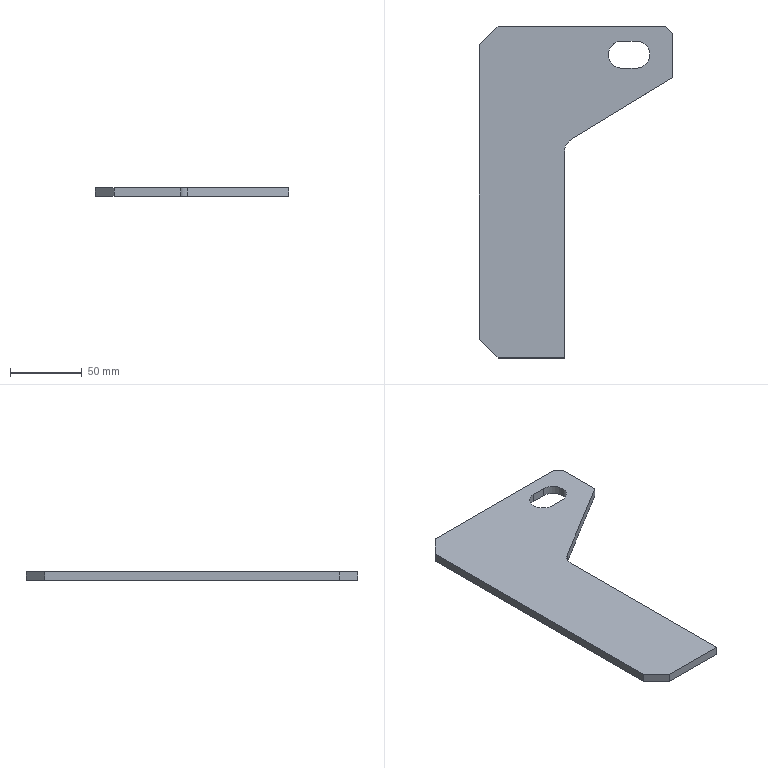Part | STEP file | 筋Plate-250×125-5 | 1 solid | 17 faces | box 135 x 232 x 6 mm | volume 105651 mm3 | plane 13 | cylinder 4 | commonest cylinder face diameters 19 x3 20 x1
STEP:
#1=CARTESIAN_POINT('',(0.,0.,0.));
#2=DIRECTION('',(0.,0.,1.));
#3=DIRECTION('',(1.,0.,0.));
#4=AXIS2_PLACEMENT_3D('',#1,#2,#3);
#5=CARTESIAN_POINT('',(32.,105.5,3.));
#6=VERTEX_POINT('',#5);
#7=CARTESIAN_POINT('',(32.,105.5,-3.));
#8=VERTEX_POINT('',#7);
#9=CARTESIAN_POINT('',(32.,105.5,-3.));
#10=DIRECTION('',(0.,0.,-1.));
#11=VECTOR('',#10,1.);
#12=LINE('',#9,#11);
#13=CARTESIAN_POINT('',(32.,96.,-3.));
#14=DIRECTION('',(0.,0.,-1.));
#15=DIRECTION('',(-1.,0.,0.));
#16=AXIS2_PLACEMENT_3D('',#13,#14,#15);
#17=CYLINDRICAL_SURFACE('',#16,9.5);
#18=CARTESIAN_POINT('',(1.571,0.));
#19=DIRECTION('',(0.,1.));
#20=VECTOR('',#19,1.);
#21=LINE('',#18,#20);
#22=(GEOMETRIC_REPRESENTATION_CONTEXT(2)PARAMETRIC_REPRESENTATION_CONTEXT()REPRESENTATION_CONTEXT('',''));
#23=DEFINITIONAL_REPRESENTATION('',(#21),#22);
#24=PCURVE('',#17,#23);
#25=CARTESIAN_POINT('',(42.,105.5,-3.));
#26=DIRECTION('',(0.,1.,0.));
#27=DIRECTION('',(0.,0.,1.));
#28=AXIS2_PLACEMENT_3D('',#25,#26,#27);
#29=PLANE('',#28);
#30=CARTESIAN_POINT('',(0.,-10.));
#31=DIRECTION('',(-1.,0.));
#32=VECTOR('',#31,1.);
#33=LINE('',#30,#32);
#34=(GEOMETRIC_REPRESENTATION_CONTEXT(2)PARAMETRIC_REPRESENTATION_CONTEXT()REPRESENTATION_CONTEXT('',''));
#35=DEFINITIONAL_REPRESENTATION('',(#33),#34);
#36=PCURVE('',#29,#35);
#37=SURFACE_CURVE('',#12,(#24,#36),.PCURVE_S1.);
#38=EDGE_CURVE('',#6,#8,#37,.T.);
#39=ORIENTED_EDGE('',*,*,#38,.T.);
#40=CARTESIAN_POINT('',(22.5,96.,-3.));
#41=VERTEX_POINT('',#40);
#42=CARTESIAN_POINT('',(32.,96.,-3.));
#43=DIRECTION('',(0.,0.,-1.));
#44=DIRECTION('',(-1.,0.,0.));
#45=AXIS2_PLACEMENT_3D('',#42,#43,#44);
#46=CIRCLE('',#45,9.5);
#47=CARTESIAN_POINT('',(0.,0.));
#48=DIRECTION('',(1.,0.));
#49=VECTOR('',#48,1.);
#50=LINE('',#47,#49);
#51=(GEOMETRIC_REPRESENTATION_CONTEXT(2)PARAMETRIC_REPRESENTATION_CONTEXT()REPRESENTATION_CONTEXT('',''));
#52=DEFINITIONAL_REPRESENTATION('',(#50),#51);
#53=PCURVE('',#17,#52);
#54=CARTESIAN_POINT('',(0.,0.,-3.));
#55=DIRECTION('',(0.,0.,1.));
#56=DIRECTION('',(1.,0.,0.));
#57=AXIS2_PLACEMENT_3D('',#54,#55,#56);
#58=PLANE('',#57);
#59=CARTESIAN_POINT('',(22.5,96.));
#60=CARTESIAN_POINT('',(22.5,112.454));
#61=CARTESIAN_POINT('',(36.75,104.227));
#62=CARTESIAN_POINT('',(51.,96.));
#63=CARTESIAN_POINT('',(36.75,87.773));
#64=CARTESIAN_POINT('',(22.5,79.546));
#65=CARTESIAN_POINT('',(22.5,96.));
#66=(BOUNDED_CURVE()B_SPLINE_CURVE(2,(#59,#60,#61,#62,#63,#64,#65),.UNSPECIFIED.,.T.,.F.)B_SPLINE_CURVE_WITH_KNOTS((1,2,2,2,2,1),(-2.094,0.,2.094,4.189,6.283,8.378),.UNSPECIFIED.)CURVE()GEOMETRIC_REPRESENTATION_ITEM()RATIONAL_B_SPLINE_CURVE((1.,0.5,1.,0.5,1.,0.5,1.))REPRESENTATION_ITEM(''));
#67=(GEOMETRIC_REPRESENTATION_CONTEXT(2)PARAMETRIC_REPRESENTATION_CONTEXT()REPRESENTATION_CONTEXT('',''));
#68=DEFINITIONAL_REPRESENTATION('',(#66),#67);
#69=PCURVE('',#58,#68);
#70=SURFACE_CURVE('',#46,(#53,#69),.PCURVE_S1.);
#71=EDGE_CURVE('',#41,#8,#70,.T.);
#72=ORIENTED_EDGE('',*,*,#71,.F.);
#73=CARTESIAN_POINT('',(22.5,96.,3.));
#74=VERTEX_POINT('',#73);
#75=CARTESIAN_POINT('',(22.5,96.,-3.));
#76=DIRECTION('',(0.,0.,-1.));
#77=VECTOR('',#76,1.);
#78=LINE('',#75,#77);
#79=CARTESIAN_POINT('',(0.,0.));
#80=DIRECTION('',(0.,1.));
#81=VECTOR('',#80,1.);
#82=LINE('',#79,#81);
#83=(GEOMETRIC_REPRESENTATION_CONTEXT(2)PARAMETRIC_REPRESENTATION_CONTEXT()REPRESENTATION_CONTEXT('',''));
#84=DEFINITIONAL_REPRESENTATION('',(#82),#83);
#85=PCURVE('',#17,#84);
#86=CARTESIAN_POINT('',(32.,96.,-3.));
#87=DIRECTION('',(0.,0.,-1.));
#88=DIRECTION('',(-1.,0.,0.));
#89=AXIS2_PLACEMENT_3D('',#86,#87,#88);
#90=CYLINDRICAL_SURFACE('',#89,9.5);
#91=CARTESIAN_POINT('',(6.283,0.));
#92=DIRECTION('',(0.,1.));
#93=VECTOR('',#92,1.);
#94=LINE('',#91,#93);
#95=(GEOMETRIC_REPRESENTATION_CONTEXT(2)PARAMETRIC_REPRESENTATION_CONTEXT()REPRESENTATION_CONTEXT('',''));
#96=DEFINITIONAL_REPRESENTATION('',(#94),#95);
#97=PCURVE('',#90,#96);
#98=SURFACE_CURVE('',#78,(#85,#97),.PCURVE_S1.);
#99=EDGE_CURVE('',#74,#41,#98,.T.);
#100=ORIENTED_EDGE('',*,*,#99,.F.);
#101=CARTESIAN_POINT('',(32.,96.,3.));
#102=DIRECTION('',(0.,0.,1.));
#103=DIRECTION('',(1.,0.,0.));
#104=AXIS2_PLACEMENT_3D('',#101,#102,#103);
#105=CIRCLE('',#104,9.5);
#106=CARTESIAN_POINT('',(3.142,-6.));
#107=DIRECTION('',(-1.,0.));
#108=VECTOR('',#107,1.);
#109=LINE('',#106,#108);
#110=(GEOMETRIC_REPRESENTATION_CONTEXT(2)PARAMETRIC_REPRESENTATION_CONTEXT()REPRESENTATION_CONTEXT('',''));
#111=DEFINITIONAL_REPRESENTATION('',(#109),#110);
#112=PCURVE('',#17,#111);
#113=CARTESIAN_POINT('',(0.,0.,3.));
#114=DIRECTION('',(0.,0.,1.));
#115=DIRECTION('',(1.,0.,0.));
#116=AXIS2_PLACEMENT_3D('',#113,#114,#115);
#117=PLANE('',#116);
#118=CARTESIAN_POINT('',(32.,96.));
#119=DIRECTION('',(1.,0.));
#120=AXIS2_PLACEMENT_2D('',#118,#119);
#121=CIRCLE('',#120,9.5);
#122=(GEOMETRIC_REPRESENTATION_CONTEXT(2)PARAMETRIC_REPRESENTATION_CONTEXT()REPRESENTATION_CONTEXT('',''));
#123=DEFINITIONAL_REPRESENTATION('',(#121),#122);
#124=PCURVE('',#117,#123);
#125=SURFACE_CURVE('',#105,(#112,#124),.PCURVE_S1.);
#126=EDGE_CURVE('',#6,#74,#125,.T.);
#127=ORIENTED_EDGE('',*,*,#126,.F.);
#128=EDGE_LOOP('',(#39,#72,#100,#127));
#129=FACE_BOUND('',#128,.F.);
#130=ADVANCED_FACE('',(#129),#17,.F.);
#131=CARTESIAN_POINT('',(67.5,80.,-3.));
#132=VERTEX_POINT('',#131);
#133=CARTESIAN_POINT('',(67.5,111.,-3.));
#134=VERTEX_POINT('',#133);
#135=CARTESIAN_POINT('',(67.5,116.,-3.));
#136=DIRECTION('',(0.,1.,0.));
#137=VECTOR('',#136,1.);
#138=LINE('',#135,#137);
#139=CARTESIAN_POINT('',(67.5,116.,3.));
#140=DIRECTION('',(-1.,0.,0.));
#141=DIRECTION('',(0.,-1.,0.));
#142=AXIS2_PLACEMENT_3D('',#139,#140,#141);
#143=PLANE('',#142);
#144=CARTESIAN_POINT('',(0.,-6.));
#145=DIRECTION('',(-1.,0.));
#146=VECTOR('',#145,1.);
#147=LINE('',#144,#146);
#148=(GEOMETRIC_REPRESENTATION_CONTEXT(2)PARAMETRIC_REPRESENTATION_CONTEXT()REPRESENTATION_CONTEXT('',''));
#149=DEFINITIONAL_REPRESENTATION('',(#147),#148);
#150=PCURVE('',#143,#149);
#151=CARTESIAN_POINT('',(67.5,116.));
#152=DIRECTION('',(0.,1.));
#153=VECTOR('',#152,1.);
#154=LINE('',#151,#153);
#155=(GEOMETRIC_REPRESENTATION_CONTEXT(2)PARAMETRIC_REPRESENTATION_CONTEXT()REPRESENTATION_CONTEXT('',''));
#156=DEFINITIONAL_REPRESENTATION('',(#154),#155);
#157=PCURVE('',#58,#156);
#158=SURFACE_CURVE('',#138,(#150,#157),.PCURVE_S1.);
#159=EDGE_CURVE('',#132,#134,#158,.T.);
#160=ORIENTED_EDGE('',*,*,#159,.T.);
#161=CARTESIAN_POINT('',(67.5,111.,3.));
#162=VERTEX_POINT('',#161);
#163=CARTESIAN_POINT('',(67.5,111.,3.));
#164=DIRECTION('',(0.,0.,1.));
#165=VECTOR('',#164,1.);
#166=LINE('',#163,#165);
#167=CARTESIAN_POINT('',(5.,0.));
#168=DIRECTION('',(0.,1.));
#169=VECTOR('',#168,1.);
#170=LINE('',#167,#169);
#171=(GEOMETRIC_REPRESENTATION_CONTEXT(2)PARAMETRIC_REPRESENTATION_CONTEXT()REPRESENTATION_CONTEXT('',''));
#172=DEFINITIONAL_REPRESENTATION('',(#170),#171);
#173=PCURVE('',#143,#172);
#174=CARTESIAN_POINT('',(62.5,116.,3.));
#175=DIRECTION('',(-0.7071,-0.7071,0.));
#176=DIRECTION('',(0.,0.,-1.));
#177=AXIS2_PLACEMENT_3D('',#174,#175,#176);
#178=PLANE('',#177);
#179=CARTESIAN_POINT('',(0.,7.071));
#180=DIRECTION('',(-1.,0.));
#181=VECTOR('',#180,1.);
#182=LINE('',#179,#181);
#183=(GEOMETRIC_REPRESENTATION_CONTEXT(2)PARAMETRIC_REPRESENTATION_CONTEXT()REPRESENTATION_CONTEXT('',''));
#184=DEFINITIONAL_REPRESENTATION('',(#182),#183);
#185=PCURVE('',#178,#184);
#186=SURFACE_CURVE('',#166,(#173,#185),.PCURVE_S1.);
#187=EDGE_CURVE('',#134,#162,#186,.T.);
#188=ORIENTED_EDGE('',*,*,#187,.T.);
#189=CARTESIAN_POINT('',(67.5,80.,3.));
#190=VERTEX_POINT('',#189);
#191=CARTESIAN_POINT('',(67.5,116.,3.));
#192=DIRECTION('',(0.,1.,0.));
#193=VECTOR('',#192,1.);
#194=LINE('',#191,#193);
#195=CARTESIAN_POINT('',(0.,0.));
#196=DIRECTION('',(-1.,0.));
#197=VECTOR('',#196,1.);
#198=LINE('',#195,#197);
#199=(GEOMETRIC_REPRESENTATION_CONTEXT(2)PARAMETRIC_REPRESENTATION_CONTEXT()REPRESENTATION_CONTEXT('',''));
#200=DEFINITIONAL_REPRESENTATION('',(#198),#199);
#201=PCURVE('',#143,#200);
#202=CARTESIAN_POINT('',(67.5,116.));
#203=DIRECTION('',(0.,1.));
#204=VECTOR('',#203,1.);
#205=LINE('',#202,#204);
#206=(GEOMETRIC_REPRESENTATION_CONTEXT(2)PARAMETRIC_REPRESENTATION_CONTEXT()REPRESENTATION_CONTEXT('',''));
#207=DEFINITIONAL_REPRESENTATION('',(#205),#206);
#208=PCURVE('',#117,#207);
#209=SURFACE_CURVE('',#194,(#201,#208),.PCURVE_S1.);
#210=EDGE_CURVE('',#190,#162,#209,.T.);
#211=ORIENTED_EDGE('',*,*,#210,.F.);
#212=CARTESIAN_POINT('',(67.5,80.,-3.));
#213=DIRECTION('',(0.,0.,1.));
#214=VECTOR('',#213,1.);
#215=LINE('',#212,#214);
#216=CARTESIAN_POINT('',(36.,-6.));
#217=DIRECTION('',(0.,1.));
#218=VECTOR('',#217,1.);
#219=LINE('',#216,#218);
#220=(GEOMETRIC_REPRESENTATION_CONTEXT(2)PARAMETRIC_REPRESENTATION_CONTEXT()REPRESENTATION_CONTEXT('',''));
#221=DEFINITIONAL_REPRESENTATION('',(#219),#220);
#222=PCURVE('',#143,#221);
#223=CARTESIAN_POINT('',(67.5,80.,-3.));
#224=DIRECTION('',(-0.5203,0.854,0.));
#225=DIRECTION('',(-0.854,-0.5203,0.));
#226=AXIS2_PLACEMENT_3D('',#223,#224,#225);
#227=PLANE('',#226);
#228=CARTESIAN_POINT('',(0.,0.));
#229=DIRECTION('',(0.,1.));
#230=VECTOR('',#229,1.);
#231=LINE('',#228,#230);
#232=(GEOMETRIC_REPRESENTATION_CONTEXT(2)PARAMETRIC_REPRESENTATION_CONTEXT()REPRESENTATION_CONTEXT('',''));
#233=DEFINITIONAL_REPRESENTATION('',(#231),#232);
#234=PCURVE('',#227,#233);
#235=SURFACE_CURVE('',#215,(#222,#234),.PCURVE_S1.);
#236=EDGE_CURVE('',#132,#190,#235,.T.);
#237=ORIENTED_EDGE('',*,*,#236,.F.);
#238=EDGE_LOOP('',(#160,#188,#211,#237));
#239=FACE_BOUND('',#238,.T.);
#240=ADVANCED_FACE('',(#239),#143,.F.);
#241=CARTESIAN_POINT('',(62.5,116.,3.));
#242=VERTEX_POINT('',#241);
#243=CARTESIAN_POINT('',(-54.5,116.,3.));
#244=VERTEX_POINT('',#243);
#245=CARTESIAN_POINT('',(-67.5,116.,3.));
#246=DIRECTION('',(-1.,0.,0.));
#247=VECTOR('',#246,1.);
#248=LINE('',#245,#247);
#249=CARTESIAN_POINT('',(-67.5,116.,3.));
#250=DIRECTION('',(0.,-1.,0.));
#251=DIRECTION('',(0.,0.,-1.));
#252=AXIS2_PLACEMENT_3D('',#249,#250,#251);
#253=PLANE('',#252);
#254=CARTESIAN_POINT('',(0.,0.));
#255=DIRECTION('',(0.,-1.));
#256=VECTOR('',#255,1.);
#257=LINE('',#254,#256);
#258=(GEOMETRIC_REPRESENTATION_CONTEXT(2)PARAMETRIC_REPRESENTATION_CONTEXT()REPRESENTATION_CONTEXT('',''));
#259=DEFINITIONAL_REPRESENTATION('',(#257),#258);
#260=PCURVE('',#253,#259);
#261=CARTESIAN_POINT('',(-67.5,116.));
#262=DIRECTION('',(-1.,0.));
#263=VECTOR('',#262,1.);
#264=LINE('',#261,#263);
#265=(GEOMETRIC_REPRESENTATION_CONTEXT(2)PARAMETRIC_REPRESENTATION_CONTEXT()REPRESENTATION_CONTEXT('',''));
#266=DEFINITIONAL_REPRESENTATION('',(#264),#265);
#267=PCURVE('',#117,#266);
#268=SURFACE_CURVE('',#248,(#260,#267),.PCURVE_S1.);
#269=EDGE_CURVE('',#242,#244,#268,.T.);
#270=ORIENTED_EDGE('',*,*,#269,.F.);
#271=CARTESIAN_POINT('',(62.5,116.,-3.));
#272=VERTEX_POINT('',#271);
#273=CARTESIAN_POINT('',(62.5,116.,3.));
#274=DIRECTION('',(0.,0.,-1.));
#275=VECTOR('',#274,1.);
#276=LINE('',#273,#275);
#277=CARTESIAN_POINT('',(0.,130.));
#278=DIRECTION('',(1.,0.));
#279=VECTOR('',#278,1.);
#280=LINE('',#277,#279);
#281=(GEOMETRIC_REPRESENTATION_CONTEXT(2)PARAMETRIC_REPRESENTATION_CONTEXT()REPRESENTATION_CONTEXT('',''));
#282=DEFINITIONAL_REPRESENTATION('',(#280),#281);
#283=PCURVE('',#253,#282);
#284=CARTESIAN_POINT('',(0.,0.));
#285=DIRECTION('',(1.,0.));
#286=VECTOR('',#285,1.);
#287=LINE('',#284,#286);
#288=(GEOMETRIC_REPRESENTATION_CONTEXT(2)PARAMETRIC_REPRESENTATION_CONTEXT()REPRESENTATION_CONTEXT('',''));
#289=DEFINITIONAL_REPRESENTATION('',(#287),#288);
#290=PCURVE('',#178,#289);
#291=SURFACE_CURVE('',#276,(#283,#290),.PCURVE_S1.);
#292=EDGE_CURVE('',#242,#272,#291,.T.);
#293=ORIENTED_EDGE('',*,*,#292,.T.);
#294=CARTESIAN_POINT('',(-54.5,116.,-3.));
#295=VERTEX_POINT('',#294);
#296=CARTESIAN_POINT('',(-67.5,116.,-3.));
#297=DIRECTION('',(-1.,0.,0.));
#298=VECTOR('',#297,1.);
#299=LINE('',#296,#298);
#300=CARTESIAN_POINT('',(6.,0.));
#301=DIRECTION('',(0.,-1.));
#302=VECTOR('',#301,1.);
#303=LINE('',#300,#302);
#304=(GEOMETRIC_REPRESENTATION_CONTEXT(2)PARAMETRIC_REPRESENTATION_CONTEXT()REPRESENTATION_CONTEXT('',''));
#305=DEFINITIONAL_REPRESENTATION('',(#303),#304);
#306=PCURVE('',#253,#305);
#307=CARTESIAN_POINT('',(-67.5,116.));
#308=DIRECTION('',(-1.,0.));
#309=VECTOR('',#308,1.);
#310=LINE('',#307,#309);
#311=(GEOMETRIC_REPRESENTATION_CONTEXT(2)PARAMETRIC_REPRESENTATION_CONTEXT()REPRESENTATION_CONTEXT('',''));
#312=DEFINITIONAL_REPRESENTATION('',(#310),#311);
#313=PCURVE('',#58,#312);
#314=SURFACE_CURVE('',#299,(#306,#313),.PCURVE_S1.);
#315=EDGE_CURVE('',#272,#295,#314,.T.);
#316=ORIENTED_EDGE('',*,*,#315,.T.);
#317=CARTESIAN_POINT('',(-54.5,116.,3.));
#318=DIRECTION('',(0.,0.,1.));
#319=VECTOR('',#318,1.);
#320=LINE('',#317,#319);
#321=CARTESIAN_POINT('',(0.,13.));
#322=DIRECTION('',(-1.,0.));
#323=VECTOR('',#322,1.);
#324=LINE('',#321,#323);
#325=(GEOMETRIC_REPRESENTATION_CONTEXT(2)PARAMETRIC_REPRESENTATION_CONTEXT()REPRESENTATION_CONTEXT('',''));
#326=DEFINITIONAL_REPRESENTATION('',(#324),#325);
#327=PCURVE('',#253,#326);
#328=CARTESIAN_POINT('',(-67.5,103.,3.));
#329=DIRECTION('',(0.7071,-0.7071,0.));
#330=DIRECTION('',(0.,0.,-1.));
#331=AXIS2_PLACEMENT_3D('',#328,#329,#330);
#332=PLANE('',#331);
#333=CARTESIAN_POINT('',(0.,18.385));
#334=DIRECTION('',(-1.,0.));
#335=VECTOR('',#334,1.);
#336=LINE('',#333,#335);
#337=(GEOMETRIC_REPRESENTATION_CONTEXT(2)PARAMETRIC_REPRESENTATION_CONTEXT()REPRESENTATION_CONTEXT('',''));
#338=DEFINITIONAL_REPRESENTATION('',(#336),#337);
#339=PCURVE('',#332,#338);
#340=SURFACE_CURVE('',#320,(#327,#339),.PCURVE_S1.);
#341=EDGE_CURVE('',#295,#244,#340,.T.);
#342=ORIENTED_EDGE('',*,*,#341,.T.);
#343=EDGE_LOOP('',(#270,#293,#316,#342));
#344=FACE_BOUND('',#343,.T.);
#345=ADVANCED_FACE('',(#344),#253,.F.);
#346=CARTESIAN_POINT('',(-67.5,103.,-3.));
#347=VERTEX_POINT('',#346);
#348=CARTESIAN_POINT('',(-67.5,-103.,-3.));
#349=VERTEX_POINT('',#348);
#350=CARTESIAN_POINT('',(-67.5,116.,-3.));
#351=DIRECTION('',(0.,-1.,0.));
#352=VECTOR('',#351,1.);
#353=LINE('',#350,#352);
#354=CARTESIAN_POINT('',(-67.5,116.,3.));
#355=DIRECTION('',(1.,0.,0.));
#356=DIRECTION('',(0.,1.,0.));
#357=AXIS2_PLACEMENT_3D('',#354,#355,#356);
#358=PLANE('',#357);
#359=CARTESIAN_POINT('',(0.,-6.));
#360=DIRECTION('',(-1.,0.));
#361=VECTOR('',#360,1.);
#362=LINE('',#359,#361);
#363=(GEOMETRIC_REPRESENTATION_CONTEXT(2)PARAMETRIC_REPRESENTATION_CONTEXT()REPRESENTATION_CONTEXT('',''));
#364=DEFINITIONAL_REPRESENTATION('',(#362),#363);
#365=PCURVE('',#358,#364);
#366=CARTESIAN_POINT('',(-67.5,116.));
#367=DIRECTION('',(0.,-1.));
#368=VECTOR('',#367,1.);
#369=LINE('',#366,#368);
#370=(GEOMETRIC_REPRESENTATION_CONTEXT(2)PARAMETRIC_REPRESENTATION_CONTEXT()REPRESENTATION_CONTEXT('',''));
#371=DEFINITIONAL_REPRESENTATION('',(#369),#370);
#372=PCURVE('',#58,#371);
#373=SURFACE_CURVE('',#353,(#365,#372),.PCURVE_S1.);
#374=EDGE_CURVE('',#347,#349,#373,.T.);
#375=ORIENTED_EDGE('',*,*,#374,.T.);
#376=CARTESIAN_POINT('',(-67.5,-103.,3.));
#377=VERTEX_POINT('',#376);
#378=CARTESIAN_POINT('',(-67.5,-103.,3.));
#379=DIRECTION('',(0.,0.,1.));
#380=VECTOR('',#379,1.);
#381=LINE('',#378,#380);
#382=CARTESIAN_POINT('',(-219.,0.));
#383=DIRECTION('',(0.,1.));
#384=VECTOR('',#383,1.);
#385=LINE('',#382,#384);
#386=(GEOMETRIC_REPRESENTATION_CONTEXT(2)PARAMETRIC_REPRESENTATION_CONTEXT()REPRESENTATION_CONTEXT('',''));
#387=DEFINITIONAL_REPRESENTATION('',(#385),#386);
#388=PCURVE('',#358,#387);
#389=CARTESIAN_POINT('',(-54.5,-116.,3.));
#390=DIRECTION('',(0.7071,0.7071,0.));
#391=DIRECTION('',(0.,0.,-1.));
#392=AXIS2_PLACEMENT_3D('',#389,#390,#391);
#393=PLANE('',#392);
#394=CARTESIAN_POINT('',(0.,18.385));
#395=DIRECTION('',(-1.,0.));
#396=VECTOR('',#395,1.);
#397=LINE('',#394,#396);
#398=(GEOMETRIC_REPRESENTATION_CONTEXT(2)PARAMETRIC_REPRESENTATION_CONTEXT()REPRESENTATION_CONTEXT('',''));
#399=DEFINITIONAL_REPRESENTATION('',(#397),#398);
#400=PCURVE('',#393,#399);
#401=SURFACE_CURVE('',#381,(#388,#400),.PCURVE_S1.);
#402=EDGE_CURVE('',#349,#377,#401,.T.);
#403=ORIENTED_EDGE('',*,*,#402,.T.);
#404=CARTESIAN_POINT('',(-67.5,103.,3.));
#405=VERTEX_POINT('',#404);
#406=CARTESIAN_POINT('',(-67.5,116.,3.));
#407=DIRECTION('',(0.,-1.,0.));
#408=VECTOR('',#407,1.);
#409=LINE('',#406,#408);
#410=CARTESIAN_POINT('',(0.,0.));
#411=DIRECTION('',(-1.,0.));
#412=VECTOR('',#411,1.);
#413=LINE('',#410,#412);
#414=(GEOMETRIC_REPRESENTATION_CONTEXT(2)PARAMETRIC_REPRESENTATION_CONTEXT()REPRESENTATION_CONTEXT('',''));
#415=DEFINITIONAL_REPRESENTATION('',(#413),#414);
#416=PCURVE('',#358,#415);
#417=CARTESIAN_POINT('',(-67.5,116.));
#418=DIRECTION('',(0.,-1.));
#419=VECTOR('',#418,1.);
#420=LINE('',#417,#419);
#421=(GEOMETRIC_REPRESENTATION_CONTEXT(2)PARAMETRIC_REPRESENTATION_CONTEXT()REPRESENTATION_CONTEXT('',''));
#422=DEFINITIONAL_REPRESENTATION('',(#420),#421);
#423=PCURVE('',#117,#422);
#424=SURFACE_CURVE('',#409,(#416,#423),.PCURVE_S1.);
#425=EDGE_CURVE('',#405,#377,#424,.T.);
#426=ORIENTED_EDGE('',*,*,#425,.F.);
#427=CARTESIAN_POINT('',(-67.5,103.,3.));
#428=DIRECTION('',(0.,0.,-1.));
#429=VECTOR('',#428,1.);
#430=LINE('',#427,#429);
#431=CARTESIAN_POINT('',(-13.,0.));
#432=DIRECTION('',(0.,-1.));
#433=VECTOR('',#432,1.);
#434=LINE('',#431,#433);
#435=(GEOMETRIC_REPRESENTATION_CONTEXT(2)PARAMETRIC_REPRESENTATION_CONTEXT()REPRESENTATION_CONTEXT('',''));
#436=DEFINITIONAL_REPRESENTATION('',(#434),#435);
#437=PCURVE('',#358,#436);
#438=CARTESIAN_POINT('',(0.,0.));
#439=DIRECTION('',(1.,0.));
#440=VECTOR('',#439,1.);
#441=LINE('',#438,#440);
#442=(GEOMETRIC_REPRESENTATION_CONTEXT(2)PARAMETRIC_REPRESENTATION_CONTEXT()REPRESENTATION_CONTEXT('',''));
#443=DEFINITIONAL_REPRESENTATION('',(#441),#442);
#444=PCURVE('',#332,#443);
#445=SURFACE_CURVE('',#430,(#437,#444),.PCURVE_S1.);
#446=EDGE_CURVE('',#405,#347,#445,.T.);
#447=ORIENTED_EDGE('',*,*,#446,.T.);
#448=EDGE_LOOP('',(#375,#403,#426,#447));
#449=FACE_BOUND('',#448,.T.);
#450=ADVANCED_FACE('',(#449),#358,.F.);
#451=CARTESIAN_POINT('',(-54.5,-116.,3.));
#452=VERTEX_POINT('',#451);
#453=CARTESIAN_POINT('',(-8.,-116.,3.));
#454=VERTEX_POINT('',#453);
#455=CARTESIAN_POINT('',(-67.5,-116.,3.));
#456=DIRECTION('',(1.,0.,0.));
#457=VECTOR('',#456,1.);
#458=LINE('',#455,#457);
#459=CARTESIAN_POINT('',(-67.5,-116.,3.));
#460=DIRECTION('',(0.,1.,0.));
#461=DIRECTION('',(0.,0.,1.));
#462=AXIS2_PLACEMENT_3D('',#459,#460,#461);
#463=PLANE('',#462);
#464=CARTESIAN_POINT('',(0.,0.));
#465=DIRECTION('',(0.,1.));
#466=VECTOR('',#465,1.);
#467=LINE('',#464,#466);
#468=(GEOMETRIC_REPRESENTATION_CONTEXT(2)PARAMETRIC_REPRESENTATION_CONTEXT()REPRESENTATION_CONTEXT('',''));
#469=DEFINITIONAL_REPRESENTATION('',(#467),#468);
#470=PCURVE('',#463,#469);
#471=CARTESIAN_POINT('',(-67.5,-116.));
#472=DIRECTION('',(1.,0.));
#473=VECTOR('',#472,1.);
#474=LINE('',#471,#473);
#475=(GEOMETRIC_REPRESENTATION_CONTEXT(2)PARAMETRIC_REPRESENTATION_CONTEXT()REPRESENTATION_CONTEXT('',''));
#476=DEFINITIONAL_REPRESENTATION('',(#474),#475);
#477=PCURVE('',#117,#476);
#478=SURFACE_CURVE('',#458,(#470,#477),.PCURVE_S1.);
#479=EDGE_CURVE('',#452,#454,#478,.T.);
#480=ORIENTED_EDGE('',*,*,#479,.F.);
#481=CARTESIAN_POINT('',(-54.5,-116.,-3.));
#482=VERTEX_POINT('',#481);
#483=CARTESIAN_POINT('',(-54.5,-116.,3.));
#484=DIRECTION('',(0.,0.,-1.));
#485=VECTOR('',#484,1.);
#486=LINE('',#483,#485);
#487=CARTESIAN_POINT('',(0.,13.));
#488=DIRECTION('',(-1.,0.));
#489=VECTOR('',#488,1.);
#490=LINE('',#487,#489);
#491=(GEOMETRIC_REPRESENTATION_CONTEXT(2)PARAMETRIC_REPRESENTATION_CONTEXT()REPRESENTATION_CONTEXT('',''));
#492=DEFINITIONAL_REPRESENTATION('',(#490),#491);
#493=PCURVE('',#463,#492);
#494=CARTESIAN_POINT('',(0.,0.));
#495=DIRECTION('',(1.,0.));
#496=VECTOR('',#495,1.);
#497=LINE('',#494,#496);
#498=(GEOMETRIC_REPRESENTATION_CONTEXT(2)PARAMETRIC_REPRESENTATION_CONTEXT()REPRESENTATION_CONTEXT('',''));
#499=DEFINITIONAL_REPRESENTATION('',(#497),#498);
#500=PCURVE('',#393,#499);
#501=SURFACE_CURVE('',#486,(#493,#500),.PCURVE_S1.);
#502=EDGE_CURVE('',#452,#482,#501,.T.);
#503=ORIENTED_EDGE('',*,*,#502,.T.);
#504=CARTESIAN_POINT('',(-8.,-116.,-3.));
#505=VERTEX_POINT('',#504);
#506=CARTESIAN_POINT('',(-67.5,-116.,-3.));
#507=DIRECTION('',(1.,0.,0.));
#508=VECTOR('',#507,1.);
#509=LINE('',#506,#508);
#510=CARTESIAN_POINT('',(-6.,0.));
#511=DIRECTION('',(0.,1.));
#512=VECTOR('',#511,1.);
#513=LINE('',#510,#512);
#514=(GEOMETRIC_REPRESENTATION_CONTEXT(2)PARAMETRIC_REPRESENTATION_CONTEXT()REPRESENTATION_CONTEXT('',''));
#515=DEFINITIONAL_REPRESENTATION('',(#513),#514);
#516=PCURVE('',#463,#515);
#517=CARTESIAN_POINT('',(-67.5,-116.));
#518=DIRECTION('',(1.,0.));
#519=VECTOR('',#518,1.);
#520=LINE('',#517,#519);
#521=(GEOMETRIC_REPRESENTATION_CONTEXT(2)PARAMETRIC_REPRESENTATION_CONTEXT()REPRESENTATION_CONTEXT('',''));
#522=DEFINITIONAL_REPRESENTATION('',(#520),#521);
#523=PCURVE('',#58,#522);
#524=SURFACE_CURVE('',#509,(#516,#523),.PCURVE_S1.);
#525=EDGE_CURVE('',#482,#505,#524,.T.);
#526=ORIENTED_EDGE('',*,*,#525,.T.);
#527=CARTESIAN_POINT('',(-8.,-116.,-3.));
#528=DIRECTION('',(0.,0.,1.));
#529=VECTOR('',#528,1.);
#530=LINE('',#527,#529);
#531=CARTESIAN_POINT('',(-6.,59.5));
#532=DIRECTION('',(1.,0.));
#533=VECTOR('',#532,1.);
#534=LINE('',#531,#533);
#535=(GEOMETRIC_REPRESENTATION_CONTEXT(2)PARAMETRIC_REPRESENTATION_CONTEXT()REPRESENTATION_CONTEXT('',''));
#536=DEFINITIONAL_REPRESENTATION('',(#534),#535);
#537=PCURVE('',#463,#536);
#538=CARTESIAN_POINT('',(-8.,-116.,-3.));
#539=DIRECTION('',(-1.,0.,0.));
#540=DIRECTION('',(0.,-1.,0.));
#541=AXIS2_PLACEMENT_3D('',#538,#539,#540);
#542=PLANE('',#541);
#543=CARTESIAN_POINT('',(0.,0.));
#544=DIRECTION('',(0.,1.));
#545=VECTOR('',#544,1.);
#546=LINE('',#543,#545);
#547=(GEOMETRIC_REPRESENTATION_CONTEXT(2)PARAMETRIC_REPRESENTATION_CONTEXT()REPRESENTATION_CONTEXT('',''));
#548=DEFINITIONAL_REPRESENTATION('',(#546),#547);
#549=PCURVE('',#542,#548);
#550=SURFACE_CURVE('',#530,(#537,#549),.PCURVE_S1.);
#551=EDGE_CURVE('',#505,#454,#550,.T.);
#552=ORIENTED_EDGE('',*,*,#551,.T.);
#553=EDGE_LOOP('',(#480,#503,#526,#552));
#554=FACE_BOUND('',#553,.T.);
#555=ADVANCED_FACE('',(#554),#463,.F.);
#556=CARTESIAN_POINT('',(32.,86.5,3.));
#557=VERTEX_POINT('',#556);
#558=CARTESIAN_POINT('',(42.,86.5,3.));
#559=VERTEX_POINT('',#558);
#560=CARTESIAN_POINT('',(0.,86.5,3.));
#561=DIRECTION('',(1.,0.,0.));
#562=VECTOR('',#561,1.);
#563=LINE('',#560,#562);
#564=CARTESIAN_POINT('',(0.,86.5));
#565=DIRECTION('',(1.,0.));
#566=VECTOR('',#565,1.);
#567=LINE('',#564,#566);
#568=(GEOMETRIC_REPRESENTATION_CONTEXT(2)PARAMETRIC_REPRESENTATION_CONTEXT()REPRESENTATION_CONTEXT('',''));
#569=DEFINITIONAL_REPRESENTATION('',(#567),#568);
#570=PCURVE('',#117,#569);
#571=CARTESIAN_POINT('',(42.,86.5,-3.));
#572=DIRECTION('',(0.,-1.,0.));
#573=DIRECTION('',(0.,0.,-1.));
#574=AXIS2_PLACEMENT_3D('',#571,#572,#573);
#575=PLANE('',#574);
#576=CARTESIAN_POINT('',(-6.,-42.));
#577=DIRECTION('',(0.,1.));
#578=VECTOR('',#577,1.);
#579=LINE('',#576,#578);
#580=(GEOMETRIC_REPRESENTATION_CONTEXT(2)PARAMETRIC_REPRESENTATION_CONTEXT()REPRESENTATION_CONTEXT('',''));
#581=DEFINITIONAL_REPRESENTATION('',(#579),#580);
#582=PCURVE('',#575,#581);
#583=SURFACE_CURVE('',#563,(#570,#582),.PCURVE_S1.);
#584=EDGE_CURVE('',#557,#559,#583,.T.);
#585=ORIENTED_EDGE('',*,*,#584,.F.);
#586=CARTESIAN_POINT('',(32.,96.,3.));
#587=DIRECTION('',(0.,0.,1.));
#588=DIRECTION('',(1.,0.,0.));
#589=AXIS2_PLACEMENT_3D('',#586,#587,#588);
#590=CIRCLE('',#589,9.5);
#591=CARTESIAN_POINT('',(32.,96.));
#592=DIRECTION('',(1.,0.));
#593=AXIS2_PLACEMENT_2D('',#591,#592);
#594=CIRCLE('',#593,9.5);
#595=(GEOMETRIC_REPRESENTATION_CONTEXT(2)PARAMETRIC_REPRESENTATION_CONTEXT()REPRESENTATION_CONTEXT('',''));
#596=DEFINITIONAL_REPRESENTATION('',(#594),#595);
#597=PCURVE('',#117,#596);
#598=CARTESIAN_POINT('',(9.425,-6.));
#599=DIRECTION('',(-1.,0.));
#600=VECTOR('',#599,1.);
#601=LINE('',#598,#600);
#602=(GEOMETRIC_REPRESENTATION_CONTEXT(2)PARAMETRIC_REPRESENTATION_CONTEXT()REPRESENTATION_CONTEXT('',''));
#603=DEFINITIONAL_REPRESENTATION('',(#601),#602);
#604=PCURVE('',#90,#603);
#605=SURFACE_CURVE('',#590,(#597,#604),.PCURVE_S1.);
#606=EDGE_CURVE('',#74,#557,#605,.T.);
#607=ORIENTED_EDGE('',*,*,#606,.F.);
#608=ORIENTED_EDGE('',*,*,#126,.F.);
#609=CARTESIAN_POINT('',(42.,105.5,3.));
#610=VERTEX_POINT('',#609);
#611=CARTESIAN_POINT('',(0.,105.5,3.));
#612=DIRECTION('',(-1.,0.,0.));
#613=VECTOR('',#612,1.);
#614=LINE('',#611,#613);
#615=CARTESIAN_POINT('',(0.,105.5));
#616=DIRECTION('',(-1.,0.));
#617=VECTOR('',#616,1.);
#618=LINE('',#615,#617);
#619=(GEOMETRIC_REPRESENTATION_CONTEXT(2)PARAMETRIC_REPRESENTATION_CONTEXT()REPRESENTATION_CONTEXT('',''));
#620=DEFINITIONAL_REPRESENTATION('',(#618),#619);
#621=PCURVE('',#117,#620);
#622=CARTESIAN_POINT('',(6.,-42.));
#623=DIRECTION('',(0.,-1.));
#624=VECTOR('',#623,1.);
#625=LINE('',#622,#624);
#626=(GEOMETRIC_REPRESENTATION_CONTEXT(2)PARAMETRIC_REPRESENTATION_CONTEXT()REPRESENTATION_CONTEXT('',''));
#627=DEFINITIONAL_REPRESENTATION('',(#625),#626);
#628=PCURVE('',#29,#627);
#629=SURFACE_CURVE('',#614,(#621,#628),.PCURVE_S1.);
#630=EDGE_CURVE('',#610,#6,#629,.T.);
#631=ORIENTED_EDGE('',*,*,#630,.F.);
#632=CARTESIAN_POINT('',(42.,96.,3.));
#633=DIRECTION('',(0.,0.,1.));
#634=DIRECTION('',(1.,0.,0.));
#635=AXIS2_PLACEMENT_3D('',#632,#633,#634);
#636=CIRCLE('',#635,9.5);
#637=CARTESIAN_POINT('',(42.,96.));
#638=DIRECTION('',(1.,0.));
#639=AXIS2_PLACEMENT_2D('',#637,#638);
#640=CIRCLE('',#639,9.5);
#641=(GEOMETRIC_REPRESENTATION_CONTEXT(2)PARAMETRIC_REPRESENTATION_CONTEXT()REPRESENTATION_CONTEXT('',''));
#642=DEFINITIONAL_REPRESENTATION('',(#640),#641);
#643=PCURVE('',#117,#642);
#644=CARTESIAN_POINT('',(42.,96.,-3.));
#645=DIRECTION('',(0.,0.,-1.));
#646=DIRECTION('',(-1.,0.,0.));
#647=AXIS2_PLACEMENT_3D('',#644,#645,#646);
#648=CYLINDRICAL_SURFACE('',#647,9.5);
#649=CARTESIAN_POINT('',(9.425,-6.));
#650=DIRECTION('',(-1.,0.));
#651=VECTOR('',#650,1.);
#652=LINE('',#649,#651);
#653=(GEOMETRIC_REPRESENTATION_CONTEXT(2)PARAMETRIC_REPRESENTATION_CONTEXT()REPRESENTATION_CONTEXT('',''));
#654=DEFINITIONAL_REPRESENTATION('',(#652),#653);
#655=PCURVE('',#648,#654);
#656=SURFACE_CURVE('',#636,(#643,#655),.PCURVE_S1.);
#657=EDGE_CURVE('',#559,#610,#656,.T.);
#658=ORIENTED_EDGE('',*,*,#657,.F.);
#659=EDGE_LOOP('',(#585,#607,#608,#631,#658));
#660=FACE_BOUND('',#659,.T.);
#661=ORIENTED_EDGE('',*,*,#210,.T.);
#662=CARTESIAN_POINT('',(89.25,89.25,3.));
#663=DIRECTION('',(-0.7071,0.7071,0.));
#664=VECTOR('',#663,1.);
#665=LINE('',#662,#664);
#666=CARTESIAN_POINT('',(89.25,89.25));
#667=DIRECTION('',(-0.7071,0.7071));
#668=VECTOR('',#667,1.);
#669=LINE('',#666,#668);
#670=(GEOMETRIC_REPRESENTATION_CONTEXT(2)PARAMETRIC_REPRESENTATION_CONTEXT()REPRESENTATION_CONTEXT('',''));
#671=DEFINITIONAL_REPRESENTATION('',(#669),#670);
#672=PCURVE('',#117,#671);
#673=CARTESIAN_POINT('',(0.,37.83));
#674=DIRECTION('',(0.,-1.));
#675=VECTOR('',#674,1.);
#676=LINE('',#673,#675);
#677=(GEOMETRIC_REPRESENTATION_CONTEXT(2)PARAMETRIC_REPRESENTATION_CONTEXT()REPRESENTATION_CONTEXT('',''));
#678=DEFINITIONAL_REPRESENTATION('',(#676),#677);
#679=PCURVE('',#178,#678);
#680=SURFACE_CURVE('',#665,(#672,#679),.PCURVE_S1.);
#681=EDGE_CURVE('',#162,#242,#680,.T.);
#682=ORIENTED_EDGE('',*,*,#681,.T.);
#683=ORIENTED_EDGE('',*,*,#269,.T.);
#684=CARTESIAN_POINT('',(-85.25,85.25,3.));
#685=DIRECTION('',(-0.7071,-0.7071,0.));
#686=VECTOR('',#685,1.);
#687=LINE('',#684,#686);
#688=CARTESIAN_POINT('',(-85.25,85.25));
#689=DIRECTION('',(-0.7071,-0.7071));
#690=VECTOR('',#689,1.);
#691=LINE('',#688,#690);
#692=(GEOMETRIC_REPRESENTATION_CONTEXT(2)PARAMETRIC_REPRESENTATION_CONTEXT()REPRESENTATION_CONTEXT('',''));
#693=DEFINITIONAL_REPRESENTATION('',(#691),#692);
#694=PCURVE('',#117,#693);
#695=CARTESIAN_POINT('',(0.,-25.102));
#696=DIRECTION('',(0.,-1.));
#697=VECTOR('',#696,1.);
#698=LINE('',#695,#697);
#699=(GEOMETRIC_REPRESENTATION_CONTEXT(2)PARAMETRIC_REPRESENTATION_CONTEXT()REPRESENTATION_CONTEXT('',''));
#700=DEFINITIONAL_REPRESENTATION('',(#698),#699);
#701=PCURVE('',#332,#700);
#702=SURFACE_CURVE('',#687,(#694,#701),.PCURVE_S1.);
#703=EDGE_CURVE('',#244,#405,#702,.T.);
#704=ORIENTED_EDGE('',*,*,#703,.T.);
#705=ORIENTED_EDGE('',*,*,#425,.T.);
#706=CARTESIAN_POINT('',(-85.25,-85.25,3.));
#707=DIRECTION('',(0.7071,-0.7071,0.));
#708=VECTOR('',#707,1.);
#709=LINE('',#706,#708);
#710=CARTESIAN_POINT('',(-85.25,-85.25));
#711=DIRECTION('',(0.7071,-0.7071));
#712=VECTOR('',#711,1.);
#713=LINE('',#710,#712);
#714=(GEOMETRIC_REPRESENTATION_CONTEXT(2)PARAMETRIC_REPRESENTATION_CONTEXT()REPRESENTATION_CONTEXT('',''));
#715=DEFINITIONAL_REPRESENTATION('',(#713),#714);
#716=PCURVE('',#117,#715);
#717=CARTESIAN_POINT('',(0.,43.487));
#718=DIRECTION('',(0.,-1.));
#719=VECTOR('',#718,1.);
#720=LINE('',#717,#719);
#721=(GEOMETRIC_REPRESENTATION_CONTEXT(2)PARAMETRIC_REPRESENTATION_CONTEXT()REPRESENTATION_CONTEXT('',''));
#722=DEFINITIONAL_REPRESENTATION('',(#720),#721);
#723=PCURVE('',#393,#722);
#724=SURFACE_CURVE('',#709,(#716,#723),.PCURVE_S1.);
#725=EDGE_CURVE('',#377,#452,#724,.T.);
#726=ORIENTED_EDGE('',*,*,#725,.T.);
#727=ORIENTED_EDGE('',*,*,#479,.T.);
#728=CARTESIAN_POINT('',(-8.,28.383,3.));
#729=VERTEX_POINT('',#728);
#730=CARTESIAN_POINT('',(-8.,-116.,3.));
#731=DIRECTION('',(0.,-1.,0.));
#732=VECTOR('',#731,1.);
#733=LINE('',#730,#732);
#734=CARTESIAN_POINT('',(-8.,-116.));
#735=DIRECTION('',(0.,-1.));
#736=VECTOR('',#735,1.);
#737=LINE('',#734,#736);
#738=(GEOMETRIC_REPRESENTATION_CONTEXT(2)PARAMETRIC_REPRESENTATION_CONTEXT()REPRESENTATION_CONTEXT('',''));
#739=DEFINITIONAL_REPRESENTATION('',(#737),#738);
#740=PCURVE('',#117,#739);
#741=CARTESIAN_POINT('',(0.,6.));
#742=DIRECTION('',(1.,0.));
#743=VECTOR('',#742,1.);
#744=LINE('',#741,#743);
#745=(GEOMETRIC_REPRESENTATION_CONTEXT(2)PARAMETRIC_REPRESENTATION_CONTEXT()REPRESENTATION_CONTEXT('',''));
#746=DEFINITIONAL_REPRESENTATION('',(#744),#745);
#747=PCURVE('',#542,#746);
#748=SURFACE_CURVE('',#733,(#740,#747),.PCURVE_S1.);
#749=EDGE_CURVE('',#729,#454,#748,.T.);
#750=ORIENTED_EDGE('',*,*,#749,.F.);
#751=CARTESIAN_POINT('',(-3.203,36.923,3.));
#752=VERTEX_POINT('',#751);
#753=CARTESIAN_POINT('',(2.,28.383,3.));
#754=DIRECTION('',(0.,0.,-1.));
#755=DIRECTION('',(1.,0.,0.));
#756=AXIS2_PLACEMENT_3D('',#753,#754,#755);
#757=CIRCLE('',#756,10.);
#758=CARTESIAN_POINT('',(12.,28.383));
#759=CARTESIAN_POINT('',(12.,11.062));
#760=CARTESIAN_POINT('',(-3.,19.723));
#761=CARTESIAN_POINT('',(-18.,28.383));
#762=CARTESIAN_POINT('',(-3.,37.043));
#763=CARTESIAN_POINT('',(12.,45.703));
#764=CARTESIAN_POINT('',(12.,28.383));
#765=(BOUNDED_CURVE()B_SPLINE_CURVE(2,(#758,#759,#760,#761,#762,#763,#764),.UNSPECIFIED.,.T.,.F.)B_SPLINE_CURVE_WITH_KNOTS((1,2,2,2,2,1),(-2.094,0.,2.094,4.189,6.283,8.378),.UNSPECIFIED.)CURVE()GEOMETRIC_REPRESENTATION_ITEM()RATIONAL_B_SPLINE_CURVE((1.,0.5,1.,0.5,1.,0.5,1.))REPRESENTATION_ITEM(''));
#766=(GEOMETRIC_REPRESENTATION_CONTEXT(2)PARAMETRIC_REPRESENTATION_CONTEXT()REPRESENTATION_CONTEXT('',''));
#767=DEFINITIONAL_REPRESENTATION('',(#765),#766);
#768=PCURVE('',#117,#767);
#769=CARTESIAN_POINT('',(2.,28.383,-3.));
#770=DIRECTION('',(0.,0.,-1.));
#771=DIRECTION('',(-1.,0.,0.));
#772=AXIS2_PLACEMENT_3D('',#769,#770,#771);
#773=CYLINDRICAL_SURFACE('',#772,10.);
#774=CARTESIAN_POINT('',(-3.142,-6.));
#775=DIRECTION('',(1.,0.));
#776=VECTOR('',#775,1.);
#777=LINE('',#774,#776);
#778=(GEOMETRIC_REPRESENTATION_CONTEXT(2)PARAMETRIC_REPRESENTATION_CONTEXT()REPRESENTATION_CONTEXT('',''));
#779=DEFINITIONAL_REPRESENTATION('',(#777),#778);
#780=PCURVE('',#773,#779);
#781=SURFACE_CURVE('',#757,(#768,#780),.PCURVE_S1.);
#782=EDGE_CURVE('',#729,#752,#781,.T.);
#783=ORIENTED_EDGE('',*,*,#782,.T.);
#784=CARTESIAN_POINT('',(67.5,80.,3.));
#785=DIRECTION('',(-0.854,-0.5203,0.));
#786=VECTOR('',#785,1.);
#787=LINE('',#784,#786);
#788=CARTESIAN_POINT('',(67.5,80.));
#789=DIRECTION('',(-0.854,-0.5203));
#790=VECTOR('',#789,1.);
#791=LINE('',#788,#790);
#792=(GEOMETRIC_REPRESENTATION_CONTEXT(2)PARAMETRIC_REPRESENTATION_CONTEXT()REPRESENTATION_CONTEXT('',''));
#793=DEFINITIONAL_REPRESENTATION('',(#791),#792);
#794=PCURVE('',#117,#793);
#795=CARTESIAN_POINT('',(0.,6.));
#796=DIRECTION('',(1.,0.));
#797=VECTOR('',#796,1.);
#798=LINE('',#795,#797);
#799=(GEOMETRIC_REPRESENTATION_CONTEXT(2)PARAMETRIC_REPRESENTATION_CONTEXT()REPRESENTATION_CONTEXT('',''));
#800=DEFINITIONAL_REPRESENTATION('',(#798),#799);
#801=PCURVE('',#227,#800);
#802=SURFACE_CURVE('',#787,(#794,#801),.PCURVE_S1.);
#803=EDGE_CURVE('',#190,#752,#802,.T.);
#804=ORIENTED_EDGE('',*,*,#803,.F.);
#805=EDGE_LOOP('',(#661,#682,#683,#704,#705,#726,#727,#750,#783,#804));
#806=FACE_BOUND('',#805,.T.);
#807=ADVANCED_FACE('',(#660,#806),#117,.T.);
#808=CARTESIAN_POINT('',(42.,105.5,-3.));
#809=VERTEX_POINT('',#808);
#810=CARTESIAN_POINT('',(42.,105.5,-3.));
#811=DIRECTION('',(-1.,0.,0.));
#812=VECTOR('',#811,1.);
#813=LINE('',#810,#812);
#814=CARTESIAN_POINT('',(42.,105.5));
#815=DIRECTION('',(-1.,0.));
#816=VECTOR('',#815,1.);
#817=LINE('',#814,#816);
#818=(GEOMETRIC_REPRESENTATION_CONTEXT(2)PARAMETRIC_REPRESENTATION_CONTEXT()REPRESENTATION_CONTEXT('',''));
#819=DEFINITIONAL_REPRESENTATION('',(#817),#818);
#820=PCURVE('',#58,#819);
#821=CARTESIAN_POINT('',(0.,0.));
#822=DIRECTION('',(0.,-1.));
#823=VECTOR('',#822,1.);
#824=LINE('',#821,#823);
#825=(GEOMETRIC_REPRESENTATION_CONTEXT(2)PARAMETRIC_REPRESENTATION_CONTEXT()REPRESENTATION_CONTEXT('',''));
#826=DEFINITIONAL_REPRESENTATION('',(#824),#825);
#827=PCURVE('',#29,#826);
#828=SURFACE_CURVE('',#813,(#820,#827),.PCURVE_S1.);
#829=EDGE_CURVE('',#809,#8,#828,.T.);
#830=ORIENTED_EDGE('',*,*,#829,.T.);
#831=ORIENTED_EDGE('',*,*,#71,.F.);
#832=CARTESIAN_POINT('',(32.,86.5,-3.));
#833=VERTEX_POINT('',#832);
#834=CARTESIAN_POINT('',(32.,96.,-3.));
#835=DIRECTION('',(0.,0.,-1.));
#836=DIRECTION('',(-1.,0.,0.));
#837=AXIS2_PLACEMENT_3D('',#834,#835,#836);
#838=CIRCLE('',#837,9.5);
#839=CARTESIAN_POINT('',(22.5,96.));
#840=CARTESIAN_POINT('',(22.5,112.454));
#841=CARTESIAN_POINT('',(36.75,104.227));
#842=CARTESIAN_POINT('',(51.,96.));
#843=CARTESIAN_POINT('',(36.75,87.773));
#844=CARTESIAN_POINT('',(22.5,79.546));
#845=CARTESIAN_POINT('',(22.5,96.));
#846=(BOUNDED_CURVE()B_SPLINE_CURVE(2,(#839,#840,#841,#842,#843,#844,#845),.UNSPECIFIED.,.T.,.F.)B_SPLINE_CURVE_WITH_KNOTS((1,2,2,2,2,1),(-2.094,0.,2.094,4.189,6.283,8.378),.UNSPECIFIED.)CURVE()GEOMETRIC_REPRESENTATION_ITEM()RATIONAL_B_SPLINE_CURVE((1.,0.5,1.,0.5,1.,0.5,1.))REPRESENTATION_ITEM(''));
#847=(GEOMETRIC_REPRESENTATION_CONTEXT(2)PARAMETRIC_REPRESENTATION_CONTEXT()REPRESENTATION_CONTEXT('',''));
#848=DEFINITIONAL_REPRESENTATION('',(#846),#847);
#849=PCURVE('',#58,#848);
#850=CARTESIAN_POINT('',(0.,0.));
#851=DIRECTION('',(1.,0.));
#852=VECTOR('',#851,1.);
#853=LINE('',#850,#852);
#854=(GEOMETRIC_REPRESENTATION_CONTEXT(2)PARAMETRIC_REPRESENTATION_CONTEXT()REPRESENTATION_CONTEXT('',''));
#855=DEFINITIONAL_REPRESENTATION('',(#853),#854);
#856=PCURVE('',#90,#855);
#857=SURFACE_CURVE('',#838,(#849,#856),.PCURVE_S1.);
#858=EDGE_CURVE('',#833,#41,#857,.T.);
#859=ORIENTED_EDGE('',*,*,#858,.F.);
#860=CARTESIAN_POINT('',(42.,86.5,-3.));
#861=VERTEX_POINT('',#860);
#862=CARTESIAN_POINT('',(42.,86.5,-3.));
#863=DIRECTION('',(-1.,0.,0.));
#864=VECTOR('',#863,1.);
#865=LINE('',#862,#864);
#866=CARTESIAN_POINT('',(42.,86.5));
#867=DIRECTION('',(-1.,0.));
#868=VECTOR('',#867,1.);
#869=LINE('',#866,#868);
#870=(GEOMETRIC_REPRESENTATION_CONTEXT(2)PARAMETRIC_REPRESENTATION_CONTEXT()REPRESENTATION_CONTEXT('',''));
#871=DEFINITIONAL_REPRESENTATION('',(#869),#870);
#872=PCURVE('',#58,#871);
#873=CARTESIAN_POINT('',(0.,0.));
#874=DIRECTION('',(0.,-1.));
#875=VECTOR('',#874,1.);
#876=LINE('',#873,#875);
#877=(GEOMETRIC_REPRESENTATION_CONTEXT(2)PARAMETRIC_REPRESENTATION_CONTEXT()REPRESENTATION_CONTEXT('',''));
#878=DEFINITIONAL_REPRESENTATION('',(#876),#877);
#879=PCURVE('',#575,#878);
#880=SURFACE_CURVE('',#865,(#872,#879),.PCURVE_S1.);
#881=EDGE_CURVE('',#861,#833,#880,.T.);
#882=ORIENTED_EDGE('',*,*,#881,.F.);
#883=CARTESIAN_POINT('',(42.,96.,-3.));
#884=DIRECTION('',(0.,0.,-1.));
#885=DIRECTION('',(-1.,0.,0.));
#886=AXIS2_PLACEMENT_3D('',#883,#884,#885);
#887=CIRCLE('',#886,9.5);
#888=CARTESIAN_POINT('',(32.5,96.));
#889=CARTESIAN_POINT('',(32.5,112.454));
#890=CARTESIAN_POINT('',(46.75,104.227));
#891=CARTESIAN_POINT('',(61.,96.));
#892=CARTESIAN_POINT('',(46.75,87.773));
#893=CARTESIAN_POINT('',(32.5,79.546));
#894=CARTESIAN_POINT('',(32.5,96.));
#895=(BOUNDED_CURVE()B_SPLINE_CURVE(2,(#888,#889,#890,#891,#892,#893,#894),.UNSPECIFIED.,.T.,.F.)B_SPLINE_CURVE_WITH_KNOTS((1,2,2,2,2,1),(-2.094,0.,2.094,4.189,6.283,8.378),.UNSPECIFIED.)CURVE()GEOMETRIC_REPRESENTATION_ITEM()RATIONAL_B_SPLINE_CURVE((1.,0.5,1.,0.5,1.,0.5,1.))REPRESENTATION_ITEM(''));
#896=(GEOMETRIC_REPRESENTATION_CONTEXT(2)PARAMETRIC_REPRESENTATION_CONTEXT()REPRESENTATION_CONTEXT('',''));
#897=DEFINITIONAL_REPRESENTATION('',(#895),#896);
#898=PCURVE('',#58,#897);
#899=CARTESIAN_POINT('',(0.,0.));
#900=DIRECTION('',(1.,0.));
#901=VECTOR('',#900,1.);
#902=LINE('',#899,#901);
#903=(GEOMETRIC_REPRESENTATION_CONTEXT(2)PARAMETRIC_REPRESENTATION_CONTEXT()REPRESENTATION_CONTEXT('',''));
#904=DEFINITIONAL_REPRESENTATION('',(#902),#903);
#905=PCURVE('',#648,#904);
#906=SURFACE_CURVE('',#887,(#898,#905),.PCURVE_S1.);
#907=EDGE_CURVE('',#809,#861,#906,.T.);
#908=ORIENTED_EDGE('',*,*,#907,.F.);
#909=EDGE_LOOP('',(#830,#831,#859,#882,#908));
#910=FACE_BOUND('',#909,.T.);
#911=ORIENTED_EDGE('',*,*,#315,.F.);
#912=CARTESIAN_POINT('',(62.5,116.,-3.));
#913=DIRECTION('',(0.7071,-0.7071,0.));
#914=VECTOR('',#913,1.);
#915=LINE('',#912,#914);
#916=CARTESIAN_POINT('',(62.5,116.));
#917=DIRECTION('',(0.7071,-0.7071));
#918=VECTOR('',#917,1.);
#919=LINE('',#916,#918);
#920=(GEOMETRIC_REPRESENTATION_CONTEXT(2)PARAMETRIC_REPRESENTATION_CONTEXT()REPRESENTATION_CONTEXT('',''));
#921=DEFINITIONAL_REPRESENTATION('',(#919),#920);
#922=PCURVE('',#58,#921);
#923=CARTESIAN_POINT('',(6.,0.));
#924=DIRECTION('',(0.,1.));
#925=VECTOR('',#924,1.);
#926=LINE('',#923,#925);
#927=(GEOMETRIC_REPRESENTATION_CONTEXT(2)PARAMETRIC_REPRESENTATION_CONTEXT()REPRESENTATION_CONTEXT('',''));
#928=DEFINITIONAL_REPRESENTATION('',(#926),#927);
#929=PCURVE('',#178,#928);
#930=SURFACE_CURVE('',#915,(#922,#929),.PCURVE_S1.);
#931=EDGE_CURVE('',#272,#134,#930,.T.);
#932=ORIENTED_EDGE('',*,*,#931,.T.);
#933=ORIENTED_EDGE('',*,*,#159,.F.);
#934=CARTESIAN_POINT('',(-3.203,36.923,-3.));
#935=VERTEX_POINT('',#934);
#936=CARTESIAN_POINT('',(67.5,80.,-3.));
#937=DIRECTION('',(-0.854,-0.5203,0.));
#938=VECTOR('',#937,1.);
#939=LINE('',#936,#938);
#940=CARTESIAN_POINT('',(67.5,80.));
#941=DIRECTION('',(-0.854,-0.5203));
#942=VECTOR('',#941,1.);
#943=LINE('',#940,#942);
#944=(GEOMETRIC_REPRESENTATION_CONTEXT(2)PARAMETRIC_REPRESENTATION_CONTEXT()REPRESENTATION_CONTEXT('',''));
#945=DEFINITIONAL_REPRESENTATION('',(#943),#944);
#946=PCURVE('',#58,#945);
#947=CARTESIAN_POINT('',(0.,0.));
#948=DIRECTION('',(1.,0.));
#949=VECTOR('',#948,1.);
#950=LINE('',#947,#949);
#951=(GEOMETRIC_REPRESENTATION_CONTEXT(2)PARAMETRIC_REPRESENTATION_CONTEXT()REPRESENTATION_CONTEXT('',''));
#952=DEFINITIONAL_REPRESENTATION('',(#950),#951);
#953=PCURVE('',#227,#952);
#954=SURFACE_CURVE('',#939,(#946,#953),.PCURVE_S1.);
#955=EDGE_CURVE('',#132,#935,#954,.T.);
#956=ORIENTED_EDGE('',*,*,#955,.T.);
#957=CARTESIAN_POINT('',(-8.,28.383,-3.));
#958=VERTEX_POINT('',#957);
#959=CARTESIAN_POINT('',(2.,28.383,-3.));
#960=DIRECTION('',(0.,0.,1.));
#961=DIRECTION('',(1.,0.,0.));
#962=AXIS2_PLACEMENT_3D('',#959,#960,#961);
#963=CIRCLE('',#962,10.);
#964=CARTESIAN_POINT('',(2.,28.383));
#965=DIRECTION('',(1.,0.));
#966=AXIS2_PLACEMENT_2D('',#964,#965);
#967=CIRCLE('',#966,10.);
#968=(GEOMETRIC_REPRESENTATION_CONTEXT(2)PARAMETRIC_REPRESENTATION_CONTEXT()REPRESENTATION_CONTEXT('',''));
#969=DEFINITIONAL_REPRESENTATION('',(#967),#968);
#970=PCURVE('',#58,#969);
#971=CARTESIAN_POINT('',(3.142,0.));
#972=DIRECTION('',(-1.,0.));
#973=VECTOR('',#972,1.);
#974=LINE('',#971,#973);
#975=(GEOMETRIC_REPRESENTATION_CONTEXT(2)PARAMETRIC_REPRESENTATION_CONTEXT()REPRESENTATION_CONTEXT('',''));
#976=DEFINITIONAL_REPRESENTATION('',(#974),#975);
#977=PCURVE('',#773,#976);
#978=SURFACE_CURVE('',#963,(#970,#977),.PCURVE_S1.);
#979=EDGE_CURVE('',#935,#958,#978,.T.);
#980=ORIENTED_EDGE('',*,*,#979,.T.);
#981=CARTESIAN_POINT('',(-8.,-116.,-3.));
#982=DIRECTION('',(0.,-1.,0.));
#983=VECTOR('',#982,1.);
#984=LINE('',#981,#983);
#985=CARTESIAN_POINT('',(-8.,-116.));
#986=DIRECTION('',(0.,-1.));
#987=VECTOR('',#986,1.);
#988=LINE('',#985,#987);
#989=(GEOMETRIC_REPRESENTATION_CONTEXT(2)PARAMETRIC_REPRESENTATION_CONTEXT()REPRESENTATION_CONTEXT('',''));
#990=DEFINITIONAL_REPRESENTATION('',(#988),#989);
#991=PCURVE('',#58,#990);
#992=CARTESIAN_POINT('',(0.,0.));
#993=DIRECTION('',(1.,0.));
#994=VECTOR('',#993,1.);
#995=LINE('',#992,#994);
#996=(GEOMETRIC_REPRESENTATION_CONTEXT(2)PARAMETRIC_REPRESENTATION_CONTEXT()REPRESENTATION_CONTEXT('',''));
#997=DEFINITIONAL_REPRESENTATION('',(#995),#996);
#998=PCURVE('',#542,#997);
#999=SURFACE_CURVE('',#984,(#991,#998),.PCURVE_S1.);
#1000=EDGE_CURVE('',#958,#505,#999,.T.);
#1001=ORIENTED_EDGE('',*,*,#1000,.T.);
#1002=ORIENTED_EDGE('',*,*,#525,.F.);
#1003=CARTESIAN_POINT('',(-54.5,-116.,-3.));
#1004=DIRECTION('',(-0.7071,0.7071,0.));
#1005=VECTOR('',#1004,1.);
#1006=LINE('',#1003,#1005);
#1007=CARTESIAN_POINT('',(-54.5,-116.));
#1008=DIRECTION('',(-0.7071,0.7071));
#1009=VECTOR('',#1008,1.);
#1010=LINE('',#1007,#1009);
#1011=(GEOMETRIC_REPRESENTATION_CONTEXT(2)PARAMETRIC_REPRESENTATION_CONTEXT()REPRESENTATION_CONTEXT('',''));
#1012=DEFINITIONAL_REPRESENTATION('',(#1010),#1011);
#1013=PCURVE('',#58,#1012);
#1014=CARTESIAN_POINT('',(6.,0.));
#1015=DIRECTION('',(0.,1.));
#1016=VECTOR('',#1015,1.);
#1017=LINE('',#1014,#1016);
#1018=(GEOMETRIC_REPRESENTATION_CONTEXT(2)PARAMETRIC_REPRESENTATION_CONTEXT()REPRESENTATION_CONTEXT('',''));
#1019=DEFINITIONAL_REPRESENTATION('',(#1017),#1018);
#1020=PCURVE('',#393,#1019);
#1021=SURFACE_CURVE('',#1006,(#1013,#1020),.PCURVE_S1.);
#1022=EDGE_CURVE('',#482,#349,#1021,.T.);
#1023=ORIENTED_EDGE('',*,*,#1022,.T.);
#1024=ORIENTED_EDGE('',*,*,#374,.F.);
#1025=CARTESIAN_POINT('',(-67.5,103.,-3.));
#1026=DIRECTION('',(0.7071,0.7071,0.));
#1027=VECTOR('',#1026,1.);
#1028=LINE('',#1025,#1027);
#1029=CARTESIAN_POINT('',(-67.5,103.));
#1030=DIRECTION('',(0.7071,0.7071));
#1031=VECTOR('',#1030,1.);
#1032=LINE('',#1029,#1031);
#1033=(GEOMETRIC_REPRESENTATION_CONTEXT(2)PARAMETRIC_REPRESENTATION_CONTEXT()REPRESENTATION_CONTEXT('',''));
#1034=DEFINITIONAL_REPRESENTATION('',(#1032),#1033);
#1035=PCURVE('',#58,#1034);
#1036=CARTESIAN_POINT('',(6.,0.));
#1037=DIRECTION('',(0.,1.));
#1038=VECTOR('',#1037,1.);
#1039=LINE('',#1036,#1038);
#1040=(GEOMETRIC_REPRESENTATION_CONTEXT(2)PARAMETRIC_REPRESENTATION_CONTEXT()REPRESENTATION_CONTEXT('',''));
#1041=DEFINITIONAL_REPRESENTATION('',(#1039),#1040);
#1042=PCURVE('',#332,#1041);
#1043=SURFACE_CURVE('',#1028,(#1035,#1042),.PCURVE_S1.);
#1044=EDGE_CURVE('',#347,#295,#1043,.T.);
#1045=ORIENTED_EDGE('',*,*,#1044,.T.);
#1046=EDGE_LOOP('',(#911,#932,#933,#956,#980,#1001,#1002,#1023,#1024,#1045));
#1047=FACE_BOUND('',#1046,.T.);
#1048=ADVANCED_FACE('',(#910,#1047),#58,.F.);
#1049=ORIENTED_EDGE('',*,*,#1000,.F.);
#1050=CARTESIAN_POINT('',(-8.,28.383,3.));
#1051=DIRECTION('',(0.,0.,1.));
#1052=VECTOR('',#1051,1.);
#1053=LINE('',#1050,#1052);
#1054=CARTESIAN_POINT('',(-144.383,6.));
#1055=DIRECTION('',(0.,1.));
#1056=VECTOR('',#1055,1.);
#1057=LINE('',#1054,#1056);
#1058=(GEOMETRIC_REPRESENTATION_CONTEXT(2)PARAMETRIC_REPRESENTATION_CONTEXT()REPRESENTATION_CONTEXT('',''));
#1059=DEFINITIONAL_REPRESENTATION('',(#1057),#1058);
#1060=PCURVE('',#542,#1059);
#1061=CARTESIAN_POINT('',(0.,-6.));
#1062=DIRECTION('',(0.,-1.));
#1063=VECTOR('',#1062,1.);
#1064=LINE('',#1061,#1063);
#1065=(GEOMETRIC_REPRESENTATION_CONTEXT(2)PARAMETRIC_REPRESENTATION_CONTEXT()REPRESENTATION_CONTEXT('',''));
#1066=DEFINITIONAL_REPRESENTATION('',(#1064),#1065);
#1067=PCURVE('',#773,#1066);
#1068=SURFACE_CURVE('',#1053,(#1060,#1067),.PCURVE_S1.);
#1069=EDGE_CURVE('',#958,#729,#1068,.T.);
#1070=ORIENTED_EDGE('',*,*,#1069,.T.);
#1071=ORIENTED_EDGE('',*,*,#749,.T.);
#1072=ORIENTED_EDGE('',*,*,#551,.F.);
#1073=EDGE_LOOP('',(#1049,#1070,#1071,#1072));
#1074=FACE_BOUND('',#1073,.T.);
#1075=ADVANCED_FACE('',(#1074),#542,.F.);
#1076=ORIENTED_EDGE('',*,*,#803,.T.);
#1077=CARTESIAN_POINT('',(-3.203,36.923,-3.));
#1078=DIRECTION('',(0.,0.,-1.));
#1079=VECTOR('',#1078,1.);
#1080=LINE('',#1077,#1079);
#1081=CARTESIAN_POINT('',(82.792,0.));
#1082=DIRECTION('',(0.,-1.));
#1083=VECTOR('',#1082,1.);
#1084=LINE('',#1081,#1083);
#1085=(GEOMETRIC_REPRESENTATION_CONTEXT(2)PARAMETRIC_REPRESENTATION_CONTEXT()REPRESENTATION_CONTEXT('',''));
#1086=DEFINITIONAL_REPRESENTATION('',(#1084),#1085);
#1087=PCURVE('',#227,#1086);
#1088=CARTESIAN_POINT('',(1.024,0.));
#1089=DIRECTION('',(0.,1.));
#1090=VECTOR('',#1089,1.);
#1091=LINE('',#1088,#1090);
#1092=(GEOMETRIC_REPRESENTATION_CONTEXT(2)PARAMETRIC_REPRESENTATION_CONTEXT()REPRESENTATION_CONTEXT('',''));
#1093=DEFINITIONAL_REPRESENTATION('',(#1091),#1092);
#1094=PCURVE('',#773,#1093);
#1095=SURFACE_CURVE('',#1080,(#1087,#1094),.PCURVE_S1.);
#1096=EDGE_CURVE('',#752,#935,#1095,.T.);
#1097=ORIENTED_EDGE('',*,*,#1096,.T.);
#1098=ORIENTED_EDGE('',*,*,#955,.F.);
#1099=ORIENTED_EDGE('',*,*,#236,.T.);
#1100=EDGE_LOOP('',(#1076,#1097,#1098,#1099));
#1101=FACE_BOUND('',#1100,.T.);
#1102=ADVANCED_FACE('',(#1101),#227,.F.);
#1103=ORIENTED_EDGE('',*,*,#725,.F.);
#1104=ORIENTED_EDGE('',*,*,#402,.F.);
#1105=ORIENTED_EDGE('',*,*,#1022,.F.);
#1106=ORIENTED_EDGE('',*,*,#502,.F.);
#1107=EDGE_LOOP('',(#1103,#1104,#1105,#1106));
#1108=FACE_BOUND('',#1107,.T.);
#1109=ADVANCED_FACE('',(#1108),#393,.F.);
#1110=ORIENTED_EDGE('',*,*,#703,.F.);
#1111=ORIENTED_EDGE('',*,*,#341,.F.);
#1112=ORIENTED_EDGE('',*,*,#1044,.F.);
#1113=ORIENTED_EDGE('',*,*,#446,.F.);
#1114=EDGE_LOOP('',(#1110,#1111,#1112,#1113));
#1115=FACE_BOUND('',#1114,.T.);
#1116=ADVANCED_FACE('',(#1115),#332,.F.);
#1117=ORIENTED_EDGE('',*,*,#681,.F.);
#1118=ORIENTED_EDGE('',*,*,#187,.F.);
#1119=ORIENTED_EDGE('',*,*,#931,.F.);
#1120=ORIENTED_EDGE('',*,*,#292,.F.);
#1121=EDGE_LOOP('',(#1117,#1118,#1119,#1120));
#1122=FACE_BOUND('',#1121,.T.);
#1123=ADVANCED_FACE('',(#1122),#178,.F.);
#1124=ORIENTED_EDGE('',*,*,#1069,.T.);
#1125=ORIENTED_EDGE('',*,*,#782,.T.);
#1126=ORIENTED_EDGE('',*,*,#1096,.T.);
#1127=ORIENTED_EDGE('',*,*,#979,.T.);
#1128=EDGE_LOOP('',(#1124,#1125,#1126,#1127));
#1129=FACE_BOUND('',#1128,.F.);
#1130=ADVANCED_FACE('',(#1129),#773,.F.);
#1131=ORIENTED_EDGE('',*,*,#858,.F.);
#1132=CARTESIAN_POINT('',(32.,86.5,-3.));
#1133=DIRECTION('',(0.,0.,1.));
#1134=VECTOR('',#1133,1.);
#1135=LINE('',#1132,#1134);
#1136=CARTESIAN_POINT('',(4.712,0.));
#1137=DIRECTION('',(0.,-1.));
#1138=VECTOR('',#1137,1.);
#1139=LINE('',#1136,#1138);
#1140=(GEOMETRIC_REPRESENTATION_CONTEXT(2)PARAMETRIC_REPRESENTATION_CONTEXT()REPRESENTATION_CONTEXT('',''));
#1141=DEFINITIONAL_REPRESENTATION('',(#1139),#1140);
#1142=PCURVE('',#90,#1141);
#1143=CARTESIAN_POINT('',(0.,-10.));
#1144=DIRECTION('',(-1.,0.));
#1145=VECTOR('',#1144,1.);
#1146=LINE('',#1143,#1145);
#1147=(GEOMETRIC_REPRESENTATION_CONTEXT(2)PARAMETRIC_REPRESENTATION_CONTEXT()REPRESENTATION_CONTEXT('',''));
#1148=DEFINITIONAL_REPRESENTATION('',(#1146),#1147);
#1149=PCURVE('',#575,#1148);
#1150=SURFACE_CURVE('',#1135,(#1142,#1149),.PCURVE_S1.);
#1151=EDGE_CURVE('',#833,#557,#1150,.T.);
#1152=ORIENTED_EDGE('',*,*,#1151,.T.);
#1153=ORIENTED_EDGE('',*,*,#606,.F.);
#1154=ORIENTED_EDGE('',*,*,#99,.T.);
#1155=EDGE_LOOP('',(#1131,#1152,#1153,#1154));
#1156=FACE_BOUND('',#1155,.F.);
#1157=ADVANCED_FACE('',(#1156),#90,.F.);
#1158=CARTESIAN_POINT('',(42.,86.5,-3.));
#1159=DIRECTION('',(0.,0.,-1.));
#1160=VECTOR('',#1159,1.);
#1161=LINE('',#1158,#1160);
#1162=CARTESIAN_POINT('',(4.712,0.));
#1163=DIRECTION('',(0.,1.));
#1164=VECTOR('',#1163,1.);
#1165=LINE('',#1162,#1164);
#1166=(GEOMETRIC_REPRESENTATION_CONTEXT(2)PARAMETRIC_REPRESENTATION_CONTEXT()REPRESENTATION_CONTEXT('',''));
#1167=DEFINITIONAL_REPRESENTATION('',(#1165),#1166);
#1168=PCURVE('',#648,#1167);
#1169=CARTESIAN_POINT('',(0.,0.));
#1170=DIRECTION('',(1.,0.));
#1171=VECTOR('',#1170,1.);
#1172=LINE('',#1169,#1171);
#1173=(GEOMETRIC_REPRESENTATION_CONTEXT(2)PARAMETRIC_REPRESENTATION_CONTEXT()REPRESENTATION_CONTEXT('',''));
#1174=DEFINITIONAL_REPRESENTATION('',(#1172),#1173);
#1175=PCURVE('',#575,#1174);
#1176=SURFACE_CURVE('',#1161,(#1168,#1175),.PCURVE_S1.);
#1177=EDGE_CURVE('',#559,#861,#1176,.T.);
#1178=ORIENTED_EDGE('',*,*,#1177,.T.);
#1179=ORIENTED_EDGE('',*,*,#907,.F.);
#1180=CARTESIAN_POINT('',(42.,105.5,-3.));
#1181=DIRECTION('',(0.,0.,1.));
#1182=VECTOR('',#1181,1.);
#1183=LINE('',#1180,#1182);
#1184=CARTESIAN_POINT('',(1.571,0.));
#1185=DIRECTION('',(0.,-1.));
#1186=VECTOR('',#1185,1.);
#1187=LINE('',#1184,#1186);
#1188=(GEOMETRIC_REPRESENTATION_CONTEXT(2)PARAMETRIC_REPRESENTATION_CONTEXT()REPRESENTATION_CONTEXT('',''));
#1189=DEFINITIONAL_REPRESENTATION('',(#1187),#1188);
#1190=PCURVE('',#648,#1189);
#1191=CARTESIAN_POINT('',(0.,0.));
#1192=DIRECTION('',(1.,0.));
#1193=VECTOR('',#1192,1.);
#1194=LINE('',#1191,#1193);
#1195=(GEOMETRIC_REPRESENTATION_CONTEXT(2)PARAMETRIC_REPRESENTATION_CONTEXT()REPRESENTATION_CONTEXT('',''));
#1196=DEFINITIONAL_REPRESENTATION('',(#1194),#1195);
#1197=PCURVE('',#29,#1196);
#1198=SURFACE_CURVE('',#1183,(#1190,#1197),.PCURVE_S1.);
#1199=EDGE_CURVE('',#809,#610,#1198,.T.);
#1200=ORIENTED_EDGE('',*,*,#1199,.T.);
#1201=ORIENTED_EDGE('',*,*,#657,.F.);
#1202=EDGE_LOOP('',(#1178,#1179,#1200,#1201));
#1203=FACE_BOUND('',#1202,.F.);
#1204=ADVANCED_FACE('',(#1203),#648,.F.);
#1205=ORIENTED_EDGE('',*,*,#630,.T.);
#1206=ORIENTED_EDGE('',*,*,#38,.T.);
#1207=ORIENTED_EDGE('',*,*,#829,.F.);
#1208=ORIENTED_EDGE('',*,*,#1199,.T.);
#1209=EDGE_LOOP('',(#1205,#1206,#1207,#1208));
#1210=FACE_BOUND('',#1209,.T.);
#1211=ADVANCED_FACE('',(#1210),#29,.F.);
#1212=ORIENTED_EDGE('',*,*,#584,.T.);
#1213=ORIENTED_EDGE('',*,*,#1177,.T.);
#1214=ORIENTED_EDGE('',*,*,#881,.T.);
#1215=ORIENTED_EDGE('',*,*,#1151,.T.);
#1216=EDGE_LOOP('',(#1212,#1213,#1214,#1215));
#1217=FACE_BOUND('',#1216,.T.);
#1218=ADVANCED_FACE('',(#1217),#575,.F.);
#1219=CLOSED_SHELL('',(#130,#240,#345,#450,#555,#807,#1048,#1075,#1102,#1109,#1116,#1123,#1130,#1157,#1204,#1211,#1218));
#1220=MANIFOLD_SOLID_BREP('',#1219);
#1221=(LENGTH_UNIT()NAMED_UNIT(*)SI_UNIT(.MILLI.,.METRE.));
#1222=UNCERTAINTY_MEASURE_WITH_UNIT(LENGTH_MEASURE(0.0000001),#1221,'','');
#1223=(NAMED_UNIT(*)PLANE_ANGLE_UNIT()SI_UNIT($,.RADIAN.));
#1224=(NAMED_UNIT(*)SI_UNIT($,.STERADIAN.)SOLID_ANGLE_UNIT());
#1225=(GEOMETRIC_REPRESENTATION_CONTEXT(3)GLOBAL_UNCERTAINTY_ASSIGNED_CONTEXT((#1222))GLOBAL_UNIT_ASSIGNED_CONTEXT((#1221,#1223,#1224))REPRESENTATION_CONTEXT('',''));
#1226=ADVANCED_BREP_SHAPE_REPRESENTATION('',(#4,#1220),#1225);